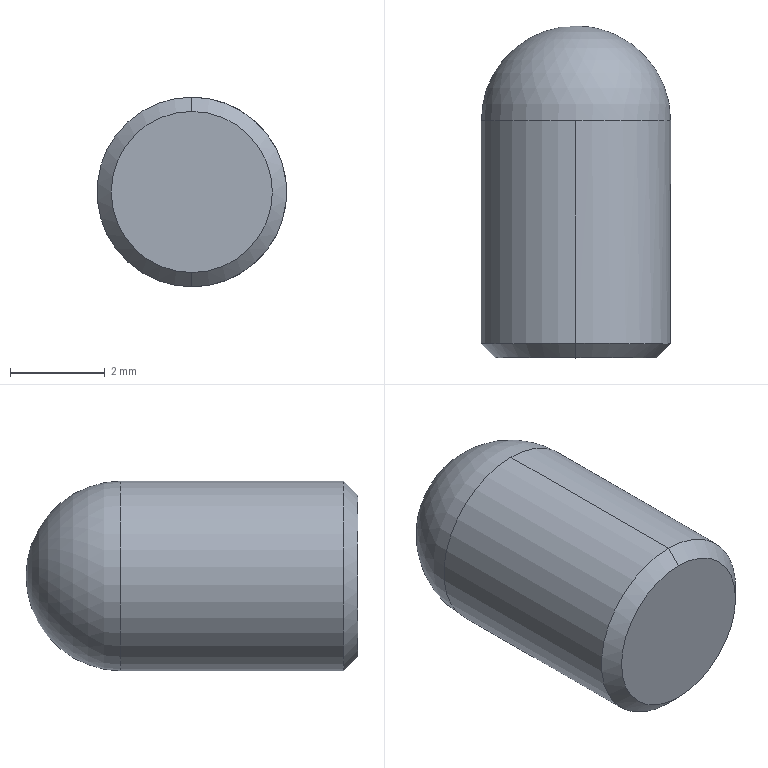Part | SolidWorks | features Chamfer 1, Dome 1, Extrusion 1 | 1 solid | 6 faces | box 4 x 7 x 4 mm | volume 79.05 mm3 | cone 2 | cylinder 2 | sphere 1 | plane 1 | commonest cylinder face diameters 4 x2
STEP:
#1=CARTESIAN_POINT('',(0.,-2.5,-1.7));
#2=VERTEX_POINT('',#1);
#3=CARTESIAN_POINT('',(0.,-2.5,1.7));
#4=VERTEX_POINT('',#3);
#5=CARTESIAN_POINT('',(0.,-2.5,0.));
#6=DIRECTION('',(0.,-1.,0.));
#7=DIRECTION('',(0.,0.,1.));
#8=AXIS2_PLACEMENT_3D('',#5,#6,#7);
#9=CIRCLE('',#8,1.7);
#10=EDGE_CURVE('',#2,#4,#9,.T.);
#11=ORIENTED_EDGE('',*,*,#10,.F.);
#12=CARTESIAN_POINT('',(0.,-2.2,-2.));
#13=VERTEX_POINT('',#12);
#14=CARTESIAN_POINT('',(0.,-2.2,-2.));
#15=DIRECTION('',(0.,0.7071,-0.7071));
#16=VECTOR('',#15,1000.);
#17=LINE('',#14,#16);
#18=EDGE_CURVE('',#2,#13,#17,.T.);
#19=ORIENTED_EDGE('',*,*,#18,.T.);
#20=CARTESIAN_POINT('',(0.,-2.2,2.));
#21=VERTEX_POINT('',#20);
#22=CARTESIAN_POINT('',(0.,-2.2,0.));
#23=DIRECTION('',(0.,1.,0.));
#24=DIRECTION('',(0.,0.,1.));
#25=AXIS2_PLACEMENT_3D('',#22,#23,#24);
#26=CIRCLE('',#25,2.);
#27=EDGE_CURVE('',#21,#13,#26,.T.);
#28=ORIENTED_EDGE('',*,*,#27,.F.);
#29=CARTESIAN_POINT('',(0.,-2.2,2.));
#30=DIRECTION('',(0.,0.7071,0.7071));
#31=VECTOR('',#30,1000.);
#32=LINE('',#29,#31);
#33=EDGE_CURVE('',#4,#21,#32,.T.);
#34=ORIENTED_EDGE('',*,*,#33,.F.);
#35=EDGE_LOOP('',(#11,#19,#28,#34));
#36=FACE_OUTER_BOUND('',#35,.T.);
#37=CARTESIAN_POINT('',(0.,-2.2,0.));
#38=DIRECTION('',(0.,1.,0.));
#39=DIRECTION('',(0.,0.,1.));
#40=AXIS2_PLACEMENT_3D('',#37,#38,#39);
#41=CONICAL_SURFACE('',#40,2.,0.7854);
#42=ADVANCED_FACE('',(#36),#41,.T.);
#43=CARTESIAN_POINT('',(0.,2.5,2.));
#44=VERTEX_POINT('',#43);
#45=CARTESIAN_POINT('',(0.,2.5,-2.));
#46=VERTEX_POINT('',#45);
#47=CARTESIAN_POINT('',(0.,2.5,0.));
#48=DIRECTION('',(0.,1.,0.));
#49=DIRECTION('',(0.,0.,1.));
#50=AXIS2_PLACEMENT_3D('',#47,#48,#49);
#51=CIRCLE('',#50,2.);
#52=EDGE_CURVE('',#44,#46,#51,.T.);
#53=ORIENTED_EDGE('',*,*,#52,.F.);
#54=CARTESIAN_POINT('',(0.,2.5,2.));
#55=DIRECTION('',(0.,-1.,0.));
#56=VECTOR('',#55,1000.);
#57=LINE('',#54,#56);
#58=EDGE_CURVE('',#44,#21,#57,.T.);
#59=ORIENTED_EDGE('',*,*,#58,.T.);
#60=ORIENTED_EDGE('',*,*,#27,.T.);
#61=CARTESIAN_POINT('',(0.,2.5,-2.));
#62=DIRECTION('',(0.,-1.,0.));
#63=VECTOR('',#62,1000.);
#64=LINE('',#61,#63);
#65=EDGE_CURVE('',#46,#13,#64,.T.);
#66=ORIENTED_EDGE('',*,*,#65,.F.);
#67=EDGE_LOOP('',(#53,#59,#60,#66));
#68=FACE_OUTER_BOUND('',#67,.T.);
#69=CARTESIAN_POINT('',(0.,2.5,0.));
#70=DIRECTION('',(0.,-1.,0.));
#71=DIRECTION('',(0.,0.,-1.));
#72=AXIS2_PLACEMENT_3D('',#69,#70,#71);
#73=CYLINDRICAL_SURFACE('',#72,2.);
#74=ADVANCED_FACE('',(#68),#73,.T.);
#75=ORIENTED_EDGE('',*,*,#58,.F.);
#76=CARTESIAN_POINT('',(0.,2.5,0.));
#77=DIRECTION('',(0.,1.,0.));
#78=DIRECTION('',(0.,0.,1.));
#79=AXIS2_PLACEMENT_3D('',#76,#77,#78);
#80=CIRCLE('',#79,2.);
#81=EDGE_CURVE('',#46,#44,#80,.T.);
#82=ORIENTED_EDGE('',*,*,#81,.F.);
#83=ORIENTED_EDGE('',*,*,#65,.T.);
#84=CARTESIAN_POINT('',(0.,-2.2,0.));
#85=DIRECTION('',(0.,1.,0.));
#86=DIRECTION('',(0.,0.,1.));
#87=AXIS2_PLACEMENT_3D('',#84,#85,#86);
#88=CIRCLE('',#87,2.);
#89=EDGE_CURVE('',#13,#21,#88,.T.);
#90=ORIENTED_EDGE('',*,*,#89,.T.);
#91=EDGE_LOOP('',(#75,#82,#83,#90));
#92=FACE_OUTER_BOUND('',#91,.T.);
#93=CARTESIAN_POINT('',(0.,2.5,0.));
#94=DIRECTION('',(0.,-1.,0.));
#95=DIRECTION('',(0.,0.,-1.));
#96=AXIS2_PLACEMENT_3D('',#93,#94,#95);
#97=CYLINDRICAL_SURFACE('',#96,2.);
#98=ADVANCED_FACE('',(#92),#97,.T.);
#99=ORIENTED_EDGE('',*,*,#81,.T.);
#100=ORIENTED_EDGE('',*,*,#52,.T.);
#101=EDGE_LOOP('',(#99,#100));
#102=FACE_OUTER_BOUND('',#101,.T.);
#103=CARTESIAN_POINT('',(0.,2.5,0.));
#104=DIRECTION('',(0.,1.,0.));
#105=DIRECTION('',(1.,0.,0.));
#106=AXIS2_PLACEMENT_3D('',#103,#104,#105);
#107=SPHERICAL_SURFACE('',#106,2.);
#108=ADVANCED_FACE('',(#102),#107,.T.);
#109=CARTESIAN_POINT('',(0.,-2.5,0.));
#110=DIRECTION('',(0.,-1.,0.));
#111=DIRECTION('',(0.,0.,1.));
#112=AXIS2_PLACEMENT_3D('',#109,#110,#111);
#113=CIRCLE('',#112,1.7);
#114=EDGE_CURVE('',#4,#2,#113,.T.);
#115=ORIENTED_EDGE('',*,*,#114,.T.);
#116=ORIENTED_EDGE('',*,*,#10,.T.);
#117=EDGE_LOOP('',(#115,#116));
#118=FACE_OUTER_BOUND('',#117,.T.);
#119=CARTESIAN_POINT('',(0.,-2.5,0.));
#120=DIRECTION('',(0.,1.,0.));
#121=DIRECTION('',(0.,0.,1.));
#122=AXIS2_PLACEMENT_3D('',#119,#120,#121);
#123=PLANE('',#122);
#124=ADVANCED_FACE('',(#118),#123,.F.);
#125=ORIENTED_EDGE('',*,*,#18,.F.);
#126=ORIENTED_EDGE('',*,*,#114,.F.);
#127=ORIENTED_EDGE('',*,*,#33,.T.);
#128=ORIENTED_EDGE('',*,*,#89,.F.);
#129=EDGE_LOOP('',(#125,#126,#127,#128));
#130=FACE_OUTER_BOUND('',#129,.T.);
#131=CARTESIAN_POINT('',(0.,-2.2,0.));
#132=DIRECTION('',(0.,1.,0.));
#133=DIRECTION('',(0.,0.,1.));
#134=AXIS2_PLACEMENT_3D('',#131,#132,#133);
#135=CONICAL_SURFACE('',#134,2.,0.7854);
#136=ADVANCED_FACE('',(#130),#135,.T.);
#137=CLOSED_SHELL('',(#42,#74,#98,#108,#124,#136));
#138=MANIFOLD_SOLID_BREP('',#137);
#139=CARTESIAN_POINT('',(0.,0.,0.));
#140=DIRECTION('',(0.,0.,1.));
#141=DIRECTION('',(1.,0.,0.));
#142=AXIS2_PLACEMENT_3D('',#139,#140,#141);
#143=(LENGTH_UNIT()NAMED_UNIT(*)SI_UNIT(.MILLI.,.METRE.));
#144=UNCERTAINTY_MEASURE_WITH_UNIT(LENGTH_MEASURE(0.00001),#143,'','');
#145=(NAMED_UNIT(*)PLANE_ANGLE_UNIT()SI_UNIT($,.RADIAN.));
#146=(NAMED_UNIT(*)SI_UNIT($,.STERADIAN.)SOLID_ANGLE_UNIT());
#147=(GEOMETRIC_REPRESENTATION_CONTEXT(3)GLOBAL_UNCERTAINTY_ASSIGNED_CONTEXT((#144))GLOBAL_UNIT_ASSIGNED_CONTEXT((#143,#145,#146))REPRESENTATION_CONTEXT('',''));
#148=ADVANCED_BREP_SHAPE_REPRESENTATION('',(#138,#142),#147);